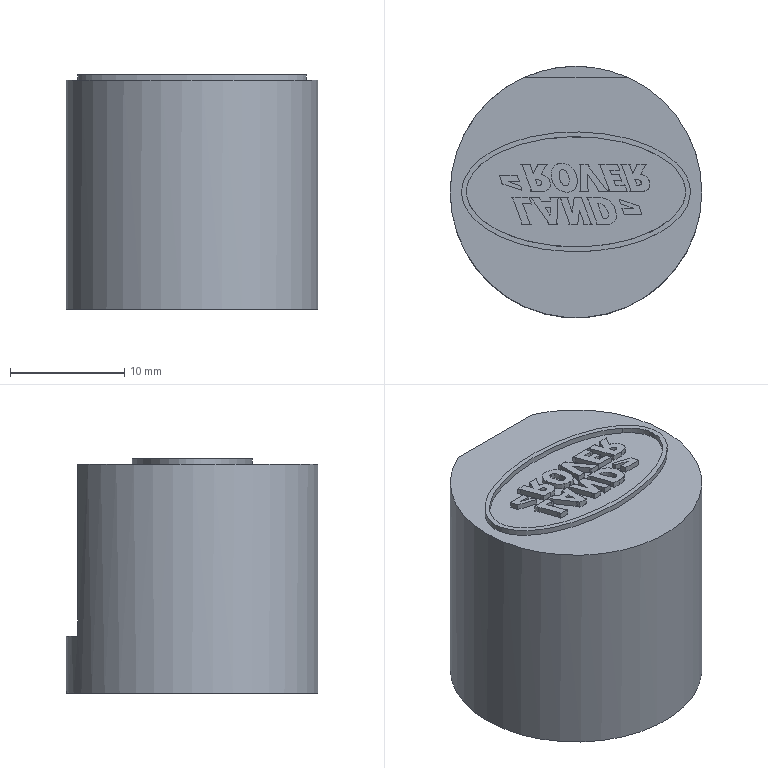Part | STEP file | lll_id686_x_t | 1 solid | 191 faces | box 22 x 22 x 20.5 mm | volume 7536 mm3 | plane 106 | other 49 | cylinder 36 | commonest cylinder face diameters 1.036 x2 0.266 x1 0.267 x1 0.399 x1 0.402 x1 0.547 x1